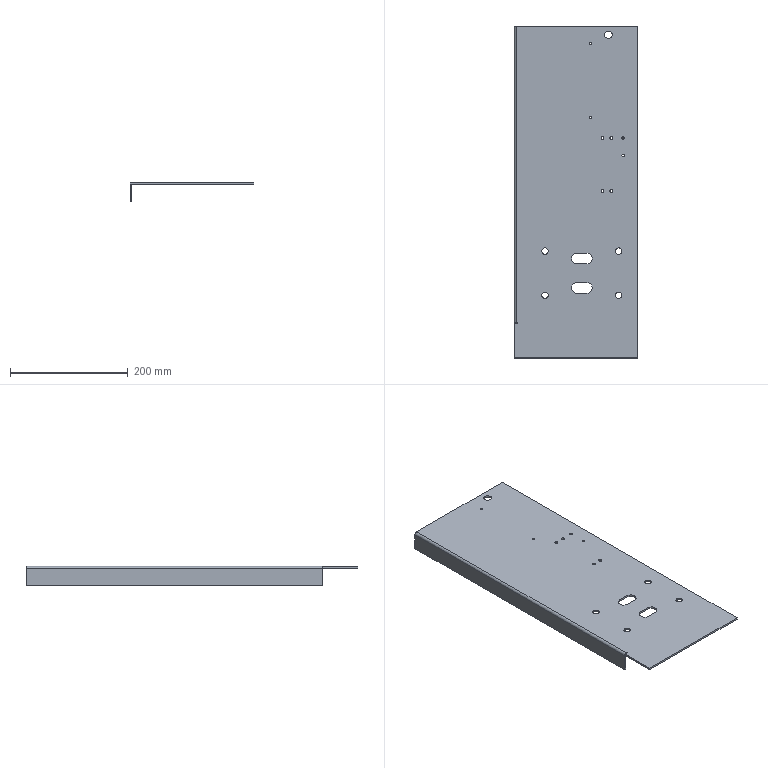Part | STEP file | PN_0005_default | 1 solid | 39 faces | box 210 x 564 x 33 mm | volume 393745 mm3 | plane 20 | cylinder 19 | commonest cylinder face diameters 4 x4 5 x4 11 x4 18 x4 2 x1 8 x1